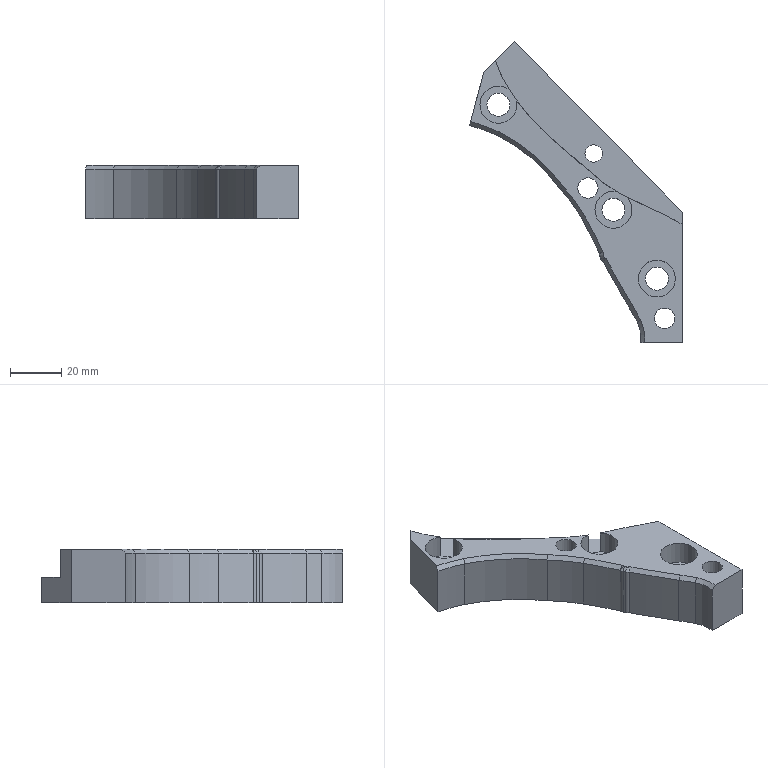Part | NX | features 23 2 | 1 solid | 43 faces | box 83.342 x 117.885 x 21 mm | volume 55345 mm3 | cylinder 18 | plane 13 | cone 10 | spline 2 | commonest cylinder face diameters 9 x3 14.5 x3 4.4 x2 8.001 x2 6.8 x1 28.064 x1